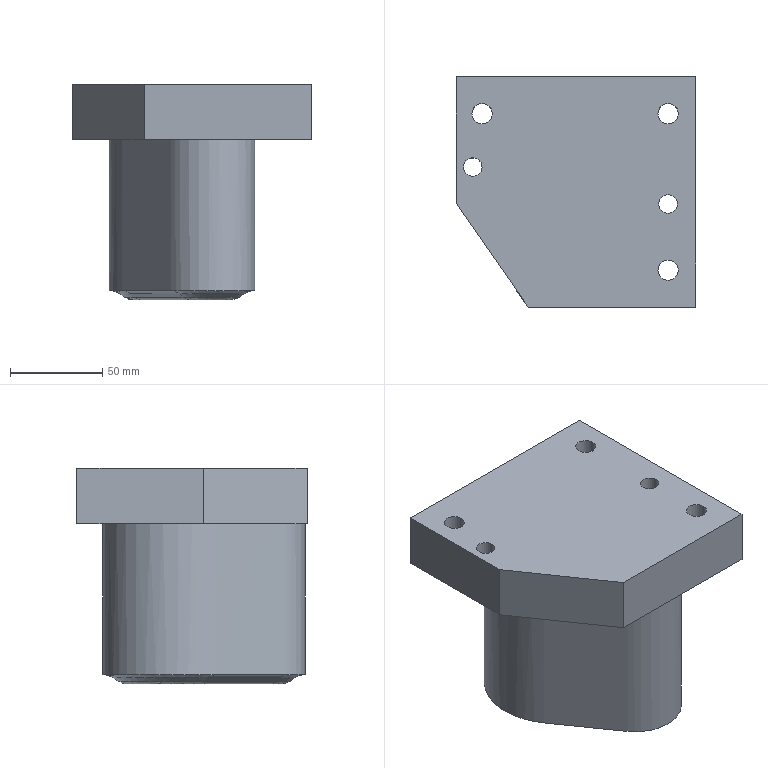Part | NX | features solid 2 | 1 solid | 32 faces | box 130 x 125 x 117 mm | volume 1005100 mm3 | spline 14 | plane 10 | cylinder 8 | commonest cylinder face diameters 11 x3 17.5 x3 10 x2